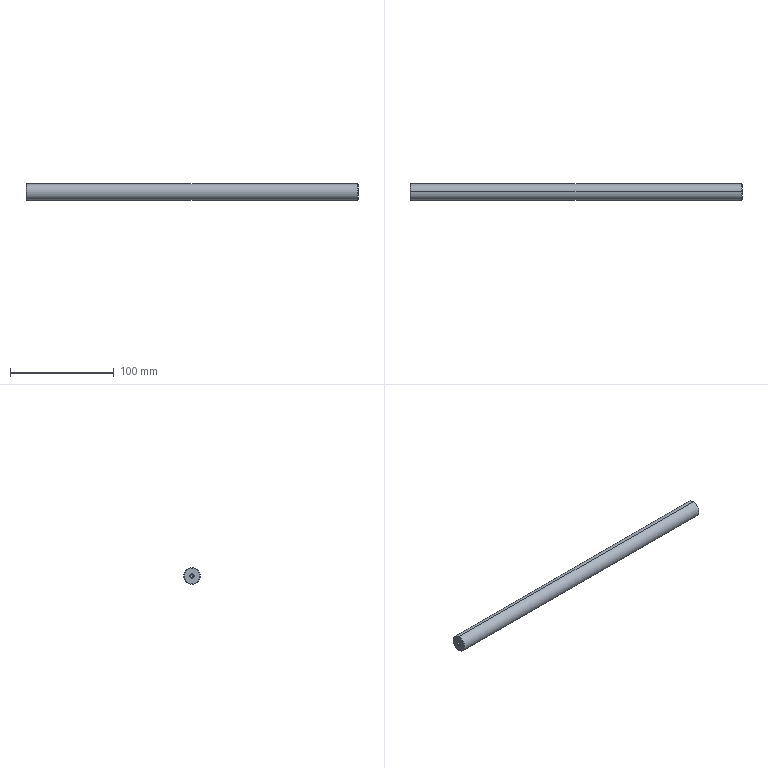Part | STEP file | 03-06 φ16 polished rod | 1 solid | 20 faces | box 320 x 16 x 16 mm | volume 64078 mm3 | cone 12 | cylinder 6 | plane 2 | commonest cylinder face diameters 3.3 x4 16 x2